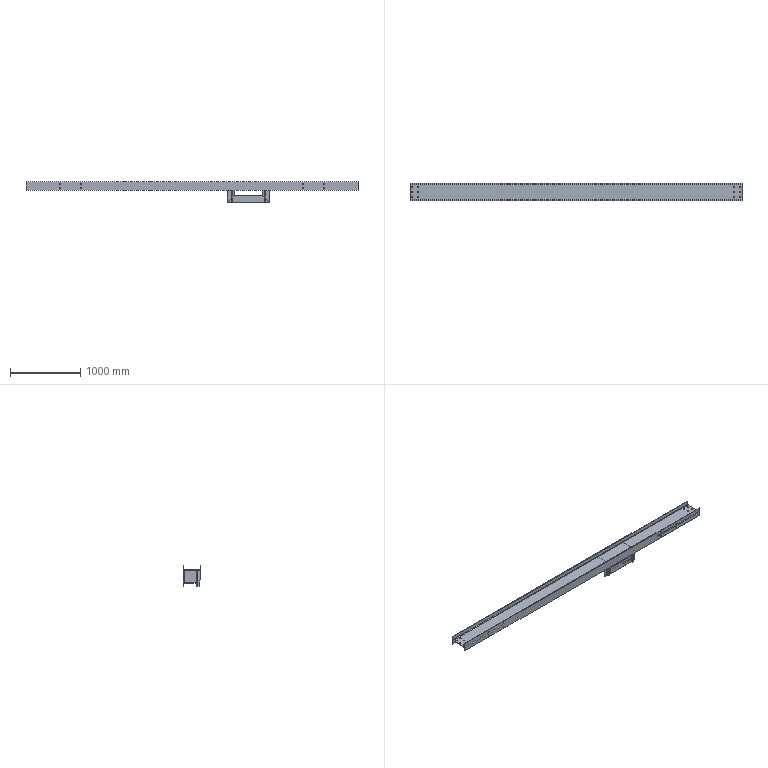Part | STEP file | 粉仓主梁1主体_Default<As Machined> | 6 solids | 138 faces | box 4730 x 250 x 295 mm | volume 19829494 mm3 | plane 82 | cylinder 56 | commonest cylinder face diameters 19 x24 15 x16 16 x16